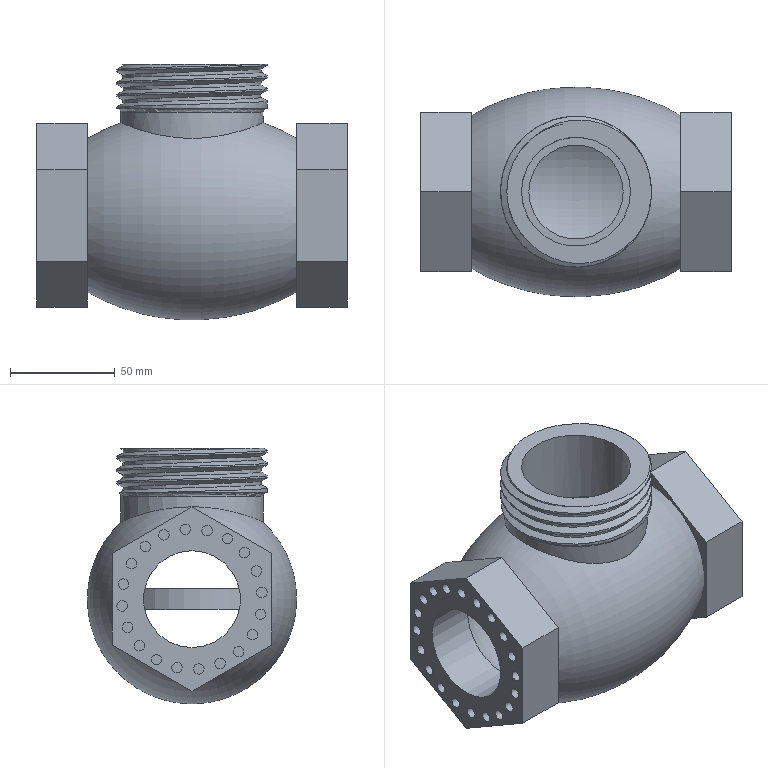Part | NX | features DATUM_CSYS 9, SKETCH 8, CYLINDER 7, EXTRUDE 6, EXTRACT_FACE 4, SYMBOLIC_THREAD 3, EXTRACT_DATUM_AXIS 2, Instance Feature 2, Mirror Feature 2, BLEND 1, CHAMFER 1, DATUM_PLANE 1, HOLE PACKAGE 1, REPLACE_FACE 1, SIMPLE HOLE 1, SWP104 1, THREADS 1 | 2 solids | 117 faces | box 148 x 100 x 122 mm | volume 413205 mm3 | plane 63 | cylinder 48 | torus 3 | spline 2 | cone 1 | commonest cylinder face diameters 5 x40 46.218 x2 68 x2 45 x1 52 x1 66 x1